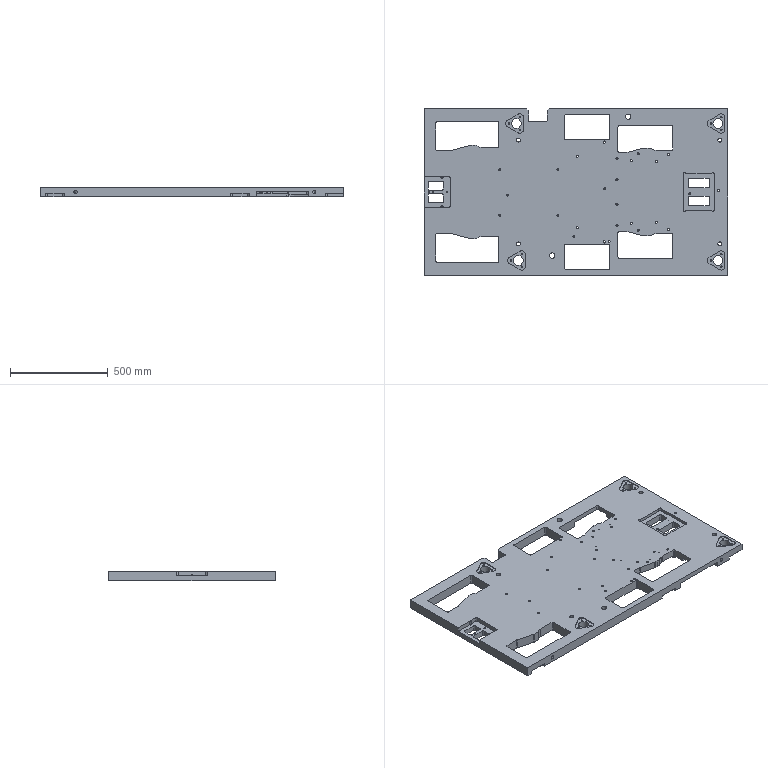Part | STEP file | lll_id3706_x_t | 1 solid | 527 faces | box 1550 x 850 x 50 mm | volume 49399285 mm3 | cylinder 242 | plane 194 | cone 75 | spline 16 | commonest cylinder face diameters 12 x49 20 x48 10.506 x20 6.8 x17 10 x16 36 x14